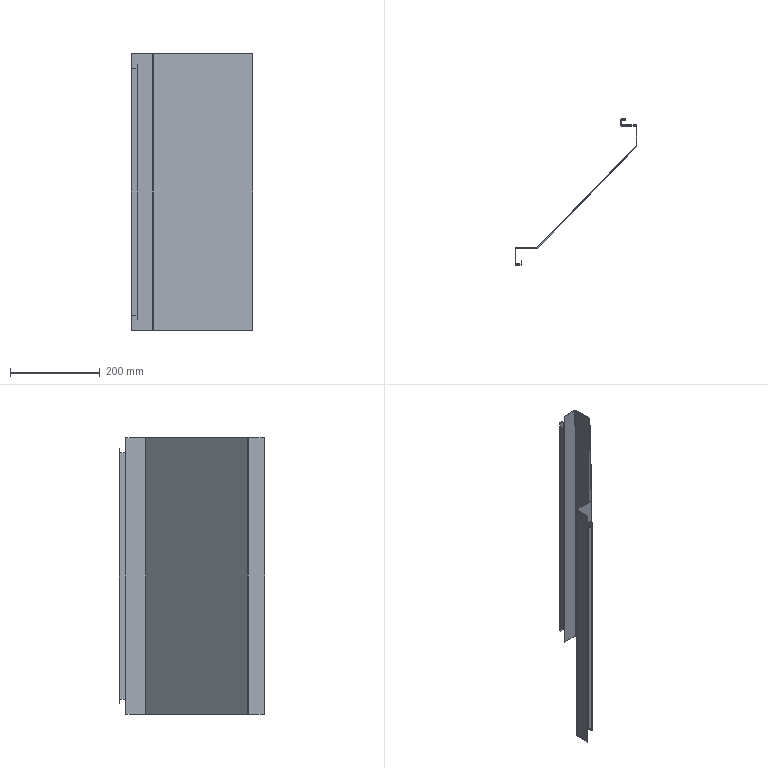Part | SolidWorks | features SMBaseFlange 3, EdgeFlange 2, Fillet 1, FlatPattern 1, SheetMetal 1 | 1 solid | 86 faces | box 272.129 x 325.286 x 617 mm | volume 483696 mm3 | plane 66 | cylinder 20 | commonest cylinder face diameters 0.2 x8 3.2 x8 10 x4